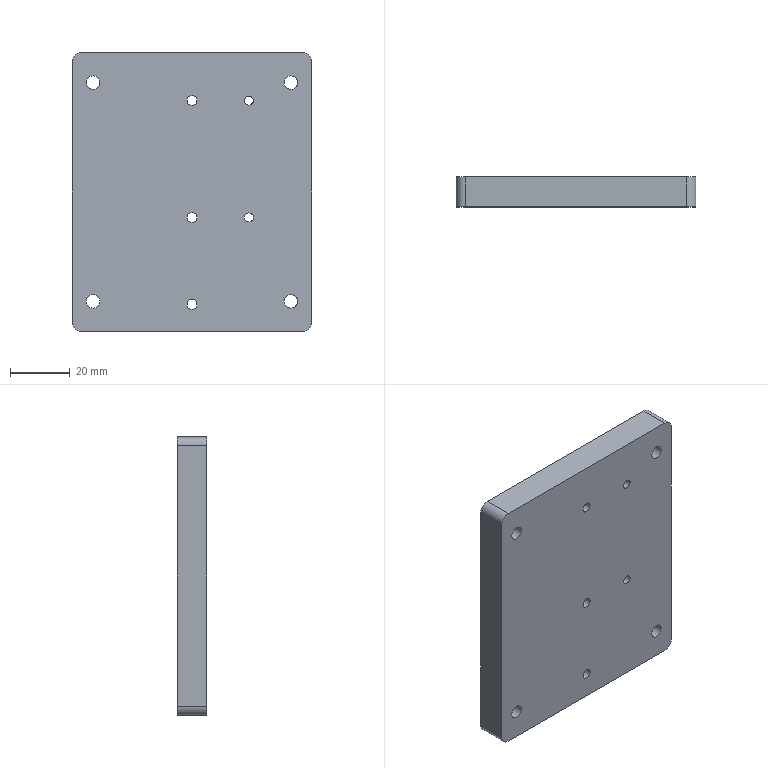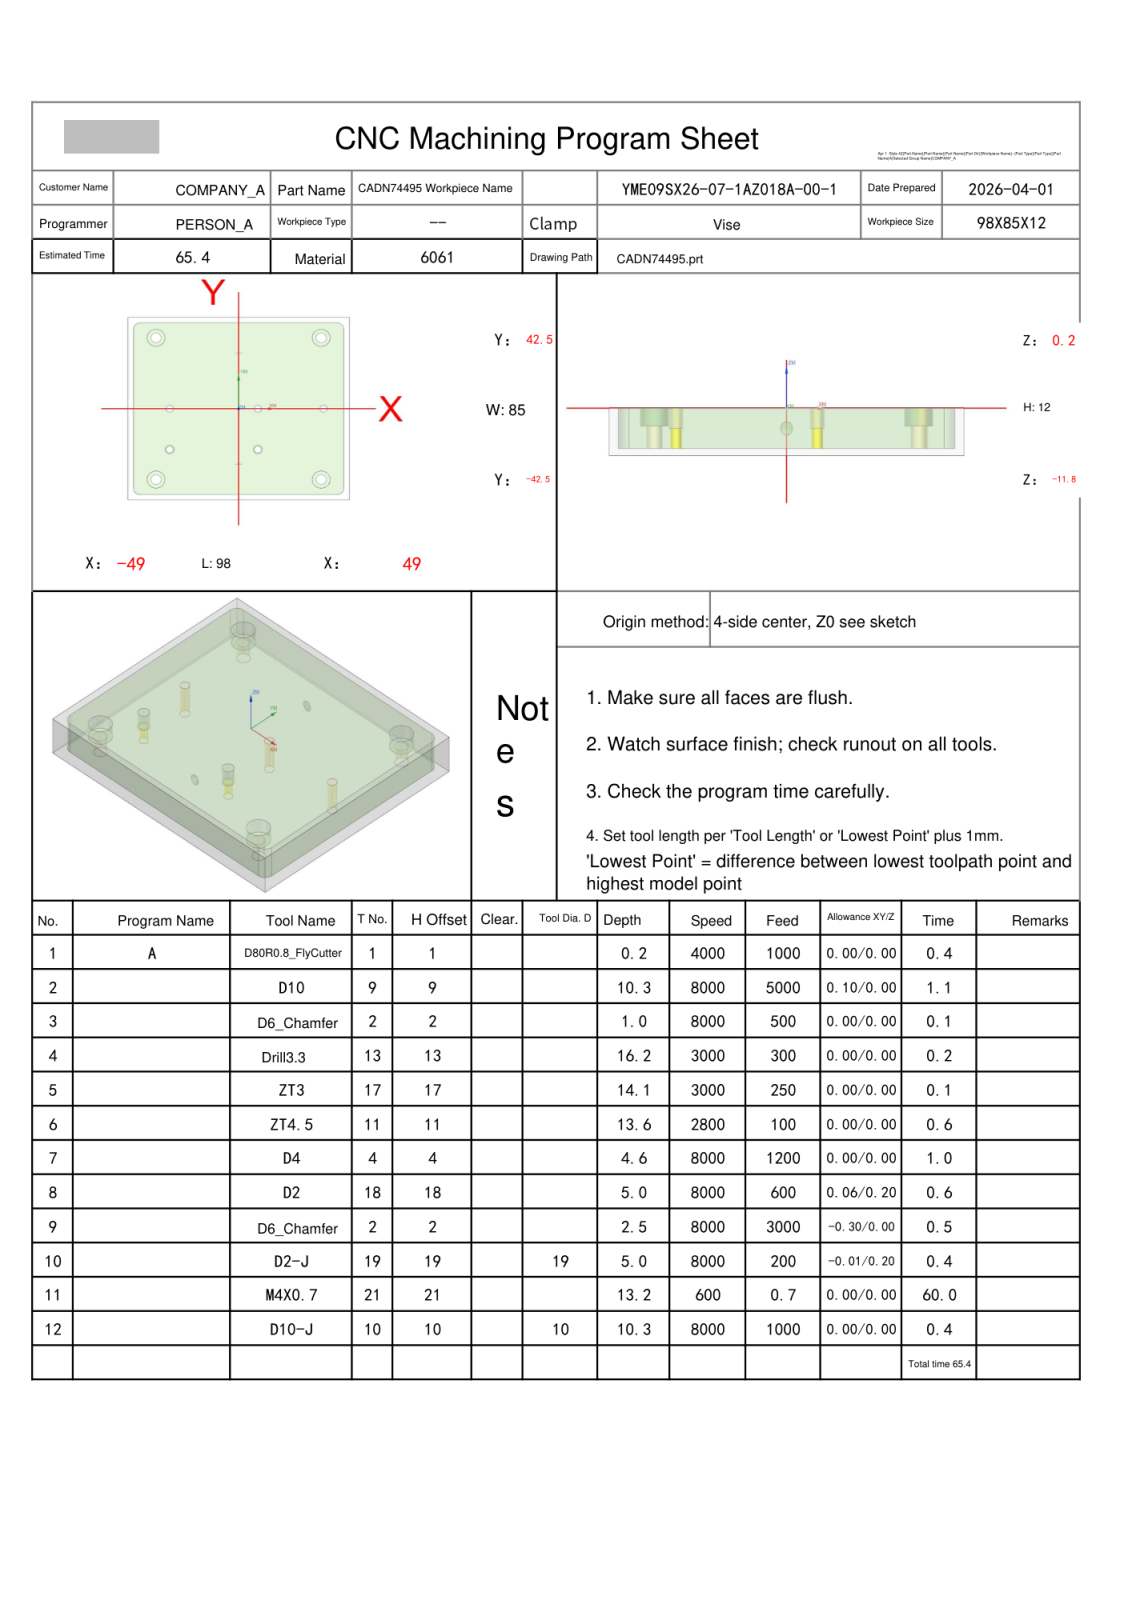NC program | NX | posted by the shop | part box 80 x 10 x 93 mm
Whole program:
%
O0001
(Machine time: 123.54 MIN)
(===Total Tool:11===)
(T1=D80R0.8 FlyCutter D=80.  R=0.8  D-  H01 Z=0.    )
(T9=D10     D=10.  R=0.   D-  H09 Z=-10.1 )
(T2=D6_Chamfer   D=6.   R=0.   D-  H02 Z=-2.3  )
(T13=Drill 3.3  D=3.3  DR_a=118 D-  H13 Z=-15.99)
(T17=ZT3    D=3.   DR_a=118 D-  H17 Z=-13.9 )
(T11=ZT4.5  D=4.5  DR_a=118 D-  H11 Z=-13.35)
(T4=D4      D=4.   R=0.   D4  H04 Z=-4.4  )
(T18=D2     D=2.   R=0.   D-  H18 Z=-4.8  )
(T19=D2-J   D=2.   R=0.   D19 H19 Z=-4.8  )
(T21=M4X0.7 D=3.3  DR_a=180 D-  H21 Z=-13.  )
(T10=D10-J  D=10.  R=0.   D10 H10 Z=-10.1 )
G80 G90 G17 G49 G40
G91 G28 Z0
M01
N1 T01 M06
(D80R0.8 FlyCutter  D=80. R=0.8 H=01 ce=0.00 di=0.00)
G00 G90 G54 X-91.5 Y26.667 M03 S4000
G43 H01 Z20.
M08
Z2.
G01 Z0.0 F1000.
X-86.5
X86.5
Y-26.667
X-86.5
X-91.5
Z2.
G00 Z20.
G91 G28 Z0.0
M05
M09
G91 G28 Z0.0
M01
N2 T09 M06
(D10  D=10. R=0. H=09 ce=0.10 di=0.00)
G00 G90 G54 X0.0 Y45.1 M03 S8000
G43 H09 Z20.
M08
Z.5
G01 X43.5 Z.412 F5000.
G02 X51.6 Y37. Z.386 I0.0 J-8.1
G01 Y-37. Z.236
G02 X43.5 Y-45.1 Z.21 I-8.1 J0.0
G01 X-43.5 Z.033
G02 X-51.6 Y-37. Z.007 I0.0 J8.1
G01 Y37. Z-.143
G02 X-43.5 Y45.1 Z-.169 I8.1 J0.0
G01 X43.5 Z-.345
G02 X51.6 Y37. Z-.371 I0.0 J-8.1
G01 Y-37. Z-.522
G02 X43.5 Y-45.1 Z-.547 I-8.1 J0.0
G01 X-43.5 Z-.724
G02 X-51.6 Y-37. Z-.75 I0.0 J8.1
G01 Y37. Z-.9
G02 X-43.5 Y45.1 Z-.926 I8.1 J0.0
G01 X43.5 Z-1.103
G02 X51.6 Y37. Z-1.128 I0.0 J-8.1
G01 Y-37. Z-1.279
G02 X43.5 Y-45.1 Z-1.305 I-8.1 J0.0
G01 X-43.5 Z-1.481
G02 X-51.6 Y-37. Z-1.507 I0.0 J8.1
G01 Y37. Z-1.657
G02 X-43.5 Y45.1 Z-1.683 I8.1 J0.0
G01 X43.5 Z-1.86
G02 X51.6 Y37. Z-1.886 I0.0 J-8.1
G01 Y-37. Z-2.036
G02 X43.5 Y-45.1 Z-2.062 I-8.1 J0.0
G01 X-43.5 Z-2.238
G02 X-51.6 Y-37. Z-2.264 I0.0 J8.1
G01 Y37. Z-2.414
G02 X-43.5 Y45.1 Z-2.44 I8.1 J0.0
G01 X43.5 Z-2.617
G02 X51.6 Y37. Z-2.643 I0.0 J-8.1
G01 Y-37. Z-2.793
G02 X43.5 Y-45.1 Z-2.819 I-8.1 J0.0
G01 X-43.5 Z-2.995
G02 X-51.6 Y-37. Z-3.021 I0.0 J8.1
G01 Y37. Z-3.172
G02 X-43.5 Y45.1 Z-3.197 I8.1 J0.0
G01 X43.5 Z-3.374
G02 X51.6 Y37. Z-3.4 I0.0 J-8.1
G01 Y-37. Z-3.55
G02 X43.5 Y-45.1 Z-3.576 I-8.1 J0.0
G01 X-43.5 Z-3.753
G02 X-51.6 Y-37. Z-3.778 I0.0 J8.1
G01 Y37. Z-3.929
G02 X-43.5 Y45.1 Z-3.955 I8.1 J0.0
G01 X43.5 Z-4.131
G02 X51.6 Y37. Z-4.157 I0.0 J-8.1
G01 Y-37. Z-4.307
G02 X43.5 Y-45.1 Z-4.333 I-8.1 J0.0
G01 X-43.5 Z-4.51
G02 X-51.6 Y-37. Z-4.536 I0.0 J8.1
G01 Y37. Z-4.686
G02 X-43.5 Y45.1 Z-4.712 I8.1 J0.0
G01 X43.5 Z-4.888
G02 X51.6 Y37. Z-4.914 I0.0 J-8.1
G01 Y-37. Z-5.064
G02 X43.5 Y-45.1 Z-5.09 I-8.1 J0.0
G01 X-43.5 Z-5.267
G02 X-51.6 Y-37. Z-5.293 I0.0 J8.1
G01 Y37. Z-5.443
G02 X-43.5 Y45.1 Z-5.469 I8.1 J0.0
G01 X43.5 Z-5.645
G02 X51.6 Y37. Z-5.671 I0.0 J-8.1
G01 Y-37. Z-5.822
G02 X43.5 Y-45.1 Z-5.847 I-8.1 J0.0
G01 X-43.5 Z-6.024
G02 X-51.6 Y-37. Z-6.05 I0.0 J8.1
G01 Y37. Z-6.2
G02 X-43.5 Y45.1 Z-6.226 I8.1 J0.0
G01 X43.5 Z-6.403
G02 X51.6 Y37. Z-6.428 I0.0 J-8.1
G01 Y-37. Z-6.579
G02 X43.5 Y-45.1 Z-6.605 I-8.1 J0.0
G01 X-43.5 Z-6.781
G02 X-51.6 Y-37. Z-6.807 I0.0 J8.1
G01 Y37. Z-6.957
G02 X-43.5 Y45.1 Z-6.983 I8.1 J0.0
G01 X43.5 Z-7.16
G02 X51.6 Y37. Z-7.186 I0.0 J-8.1
G01 Y-37. Z-7.336
G02 X43.5 Y-45.1 Z-7.362 I-8.1 J0.0
G01 X-43.5 Z-7.538
G02 X-51.6 Y-37. Z-7.564 I0.0 J8.1
G01 Y37. Z-7.714
G02 X-43.5 Y45.1 Z-7.74 I8.1 J0.0
G01 X43.5 Z-7.917
G02 X51.6 Y37. Z-7.943 I0.0 J-8.1
G01 Y-37. Z-8.093
G02 X43.5 Y-45.1 Z-8.119 I-8.1 J0.0
G01 X-43.5 Z-8.295
G02 X-51.6 Y-37. Z-8.321 I0.0 J8.1
G01 Y37. Z-8.472
G02 X-43.5 Y45.1 Z-8.497 I8.1 J0.0
G01 X43.5 Z-8.674
G02 X51.6 Y37. Z-8.7 I0.0 J-8.1
G01 Y-37. Z-8.85
G02 X43.5 Y-45.1 Z-8.876 I-8.1 J0.0
G01 X-43.5 Z-9.053
G02 X-51.6 Y-37. Z-9.078 I0.0 J8.1
G01 Y37. Z-9.229
G02 X-43.5 Y45.1 Z-9.255 I8.1 J0.0
G01 X43.5 Z-9.431
G02 X51.6 Y37. Z-9.457 I0.0 J-8.1
G01 Y-37. Z-9.607
G02 X43.5 Y-45.1 Z-9.633 I-8.1 J0.0
G01 X-43.5 Z-9.81
G02 X-51.6 Y-37. Z-9.836 I0.0 J8.1
G01 Y37. Z-9.986
G02 X-43.5 Y45.1 Z-10.012 I8.1 J0.0
G01 X0.0 Z-10.1
X43.5
G02 X51.6 Y37. I0.0 J-8.1
G01 Y-37.
G02 X43.5 Y-45.1 I-8.1 J0.0
G01 X-43.5
G02 X-51.6 Y-37. I0.0 J8.1
G01 Y37.
G02 X-43.5 Y45.1 I8.1 J0.0
G01 X0.0
X.5
Z-9.1
G00 Z20.
G91 G28 Z0.0
M05
M09
G91 G28 Z0.0
M01
N3 T02 M06
(D6_Chamfer  D=6. R=0. H=02 ce=0.00 di=0.00)
G00 G90 G54 X-36.5 Y33. M03 S8000
G43 H02 Z20.
M08
G98 G81 X-36.5 Y33. Z-.8 R1. F500.
X-30.5 Y0.0
Y-19.
X-36.5 Y-33.
X8.5 Y0.0
Y-19.
X36.5 Y-33.
X37.5 Y0.0
X36.5 Y33.
G80
G00 Z20.
G91 G28 Z0.0
M05
M09
G91 G28 Z0.0
M01
N4 T13 M06
(Drill 3.3 D=3.3 DR_a=118 H=13)
G00 G90 G54 X-30.5 Y0.0 M03 S3000
G43 H13 Z20.
M08
G98 G83 X-30.5 Y0.0 Z-15.991 R1. F300. Q2.
X8.5
X37.5
G80
G00 Z20.
G91 G28 Z0.0
M05
M09
G91 G28 Z0.0
M01
N5 T17 M06
(ZT3 D=3. DR_a=118 H=17)
G00 G90 G54 X8.5 Y-19. M03 S3000
G43 H17 Z20.
M08
G98 G83 X8.5 Y-19. Z-13.901 R1. F250. Q2.
X-30.5
G80
G00 Z20.
G91 G28 Z0.0
M05
M09
G91 G28 Z0.0
M01
N6 T11 M06
(ZT4.5 D=4.5 DR_a=118 H=11)
G00 G90 G54 X36.5 Y33. M03 S2800
G43 H11 Z20.
M08
G98 G83 X36.5 Y33. Z-13.352 R1. F100. Q2.
Y-33.
X-36.5
Y33.
G80
G00 Z20.
G91 G28 Z0.0
M05
M09
G91 G28 Z0.0
M01
N7 T04 M06
(D4  D=4. R=0. H=04 ce=0.10 di=0.00)
G00 G90 G54 X36.5 Y33. M03 S8000
G43 H04 Z20.
M08
Z.5
G03 X35.55 Y33.95 I-.95 J0.0 F1200.
X34.6 Y33. I0.0 J-.95
X34.6 Y33. Z.2 I1.9 J0.0
X34.6 Y33. Z-.1 I1.9 J0.0
X34.6 Y33. Z-.4 I1.9 J0.0
X34.6 Y33. Z-.7 I1.9 J0.0
X34.6 Y33. Z-1. I1.9 J0.0
X34.6 Y33. Z-1.3 I1.9 J0.0
X34.6 Y33. Z-1.6 I1.9 J0.0
X34.6 Y33. Z-1.9 I1.9 J0.0
X34.6 Y33. Z-2.2 I1.9 J0.0
X34.6 Y33. Z-2.5 I1.9 J0.0
X34.6 Y33. Z-2.8 I1.9 J0.0
X34.6 Y33. Z-3.1 I1.9 J0.0
X34.6 Y33. Z-3.4 I1.9 J0.0
X34.6 Y33. Z-3.7 I1.9 J0.0
X34.6 Y33. Z-4. I1.9 J0.0
X34.6 Y33. Z-4.3 I1.9 J0.0
X37.45 Y31.355 Z-4.4 I1.9 J0.0
X38.4 Y33. I-.95 J1.645
X36.5 Y34.9 I-1.9 J0.0
X34.6 Y33. I0.0 J-1.9
X36.5 Y31.1 I1.9 J0.0
X37.45 Y31.355 I0.0 J1.9
X37.925 Y32.177 I-.475 J.823
X36.975 Y33.127 I-.95 J0.0
X36.5 Y33. I0.0 J-.95
G00 Z20.
Y-33.
Z.5
G03 X35.55 Y-32.05 I-.95 J0.0
X34.6 Y-33. I0.0 J-.95
X34.6 Y-33. Z.2 I1.9 J0.0
X34.6 Y-33. Z-.1 I1.9 J0.0
X34.6 Y-33. Z-.4 I1.9 J0.0
X34.6 Y-33. Z-.7 I1.9 J0.0
X34.6 Y-33. Z-1. I1.9 J0.0
X34.6 Y-33. Z-1.3 I1.9 J0.0
X34.6 Y-33. Z-1.6 I1.9 J0.0
X34.6 Y-33. Z-1.9 I1.9 J0.0
X34.6 Y-33. Z-2.2 I1.9 J0.0
X34.6 Y-33. Z-2.5 I1.9 J0.0
X34.6 Y-33. Z-2.8 I1.9 J0.0
X34.6 Y-33. Z-3.1 I1.9 J0.0
X34.6 Y-33. Z-3.4 I1.9 J0.0
X34.6 Y-33. Z-3.7 I1.9 J0.0
X34.6 Y-33. Z-4. I1.9 J0.0
X34.6 Y-33. Z-4.3 I1.9 J0.0
X37.45 Y-34.646 Z-4.4 I1.9 J0.0
X38.4 Y-33. I-.95 J1.645
X36.5 Y-31.1 I-1.9 J0.0
X34.6 Y-33. I0.0 J-1.9
X36.5 Y-34.9 I1.9 J0.0
X37.45 Y-34.646 I0.0 J1.9
X37.925 Y-33.823 I-.475 J.823
X36.975 Y-32.873 I-.95 J0.0
X36.5 Y-33. I0.0 J-.95
G00 Z20.
X-36.5
Z.5
G03 X-37.45 Y-32.05 I-.95 J0.0
X-38.4 Y-33. I0.0 J-.95
X-38.4 Y-33. Z.2 I1.9 J0.0
X-38.4 Y-33. Z-.1 I1.9 J0.0
X-38.4 Y-33. Z-.4 I1.9 J0.0
X-38.4 Y-33. Z-.7 I1.9 J0.0
X-38.4 Y-33. Z-1. I1.9 J0.0
X-38.4 Y-33. Z-1.3 I1.9 J0.0
X-38.4 Y-33. Z-1.6 I1.9 J0.0
X-38.4 Y-33. Z-1.9 I1.9 J0.0
X-38.4 Y-33. Z-2.2 I1.9 J0.0
X-38.4 Y-33. Z-2.5 I1.9 J0.0
X-38.4 Y-33. Z-2.8 I1.9 J0.0
X-38.4 Y-33. Z-3.1 I1.9 J0.0
X-38.4 Y-33. Z-3.4 I1.9 J0.0
X-38.4 Y-33. Z-3.7 I1.9 J0.0
X-38.4 Y-33. Z-4. I1.9 J0.0
X-38.4 Y-33. Z-4.3 I1.9 J0.0
X-35.55 Y-34.646 Z-4.4 I1.9 J0.0
X-34.6 Y-33. I-.95 J1.645
X-36.5 Y-31.1 I-1.9 J0.0
X-38.4 Y-33. I0.0 J-1.9
X-36.5 Y-34.9 I1.9 J0.0
X-35.55 Y-34.646 I0.0 J1.9
X-35.075 Y-33.823 I-.475 J.823
X-36.025 Y-32.873 I-.95 J0.0
X-36.5 Y-33. I0.0 J-.95
G00 Z20.
Y33.
Z.5
G03 X-37.45 Y33.95 I-.95 J0.0
X-38.4 Y33. I0.0 J-.95
X-38.4 Y33. Z.2 I1.9 J0.0
X-38.4 Y33. Z-.1 I1.9 J0.0
X-38.4 Y33. Z-.4 I1.9 J0.0
X-38.4 Y33. Z-.7 I1.9 J0.0
X-38.4 Y33. Z-1. I1.9 J0.0
X-38.4 Y33. Z-1.3 I1.9 J0.0
X-38.4 Y33. Z-1.6 I1.9 J0.0
X-38.4 Y33. Z-1.9 I1.9 J0.0
X-38.4 Y33. Z-2.2 I1.9 J0.0
X-38.4 Y33. Z-2.5 I1.9 J0.0
X-38.4 Y33. Z-2.8 I1.9 J0.0
X-38.4 Y33. Z-3.1 I1.9 J0.0
X-38.4 Y33. Z-3.4 I1.9 J0.0
X-38.4 Y33. Z-3.7 I1.9 J0.0
X-38.4 Y33. Z-4. I1.9 J0.0
X-38.4 Y33. Z-4.3 I1.9 J0.0
X-35.55 Y31.355 Z-4.4 I1.9 J0.0
X-34.6 Y33. I-.95 J1.645
X-36.5 Y34.9 I-1.9 J0.0
X-38.4 Y33. I0.0 J-1.9
X-36.5 Y31.1 I1.9 J0.0
X-35.55 Y31.355 I0.0 J1.9
X-35.075 Y32.177 I-.475 J.823
X-36.025 Y33.127 I-.95 J0.0
X-36.5 Y33. I0.0 J-.95
G00 Z20.
G00 G90 X36.5 Y33. M03 S8000
Z20.
Z.5
G41 D04
G01 X36.46 Y33.196 F500.
G03 X35.49 Y33.99 I-.97 J-.196
X34.5 Y33. I0.0 J-.99
X34.516 Y33.251 Z-4.4 I2. J0.0
X34.5 Y33. I1.984 J-.251
X36.5 Y31. I2. J0.0
X38.5 Y33. I0.0 J2.
X36.5 Y35. I-2. J0.0
X34.516 Y33.251 I0.0 J-2.
G01 X34.508 Y33.127
G03 X35.498 Y32.137 I.99 J0.0
X36.436 Y32.81 I0.0 J.99
G01 G40 X36.5 Y33.
G00 Z20.
Y-33.
Z.5
G41 D04
G01 X36.46 Y-32.804
G03 X35.49 Y-32.01 I-.97 J-.196
X34.5 Y-33. I0.0 J-.99
X34.516 Y-32.749 Z-4.4 I2. J0.0
X34.5 Y-33. I1.984 J-.251
X36.5 Y-35. I2. J0.0
X38.5 Y-33. I0.0 J2.
X36.5 Y-31. I-2. J0.0
X34.516 Y-32.749 I0.0 J-2.
G01 X34.508 Y-32.873
G03 X35.498 Y-33.863 I.99 J0.0
X36.436 Y-33.19 I0.0 J.99
G01 G40 X36.5 Y-33.
G00 Z20.
X-36.5
Z.5
G41 D04
G01 X-36.54 Y-32.804
G03 X-37.51 Y-32.01 I-.97 J-.196
X-38.5 Y-33. I0.0 J-.99
X-38.484 Y-32.749 Z-4.4 I2. J0.0
X-38.5 Y-33. I1.984 J-.251
X-36.5 Y-35. I2. J0.0
X-34.5 Y-33. I0.0 J2.
X-36.5 Y-31. I-2. J0.0
X-38.484 Y-32.749 I0.0 J-2.
G01 X-38.492 Y-32.873
G03 X-37.502 Y-33.863 I.99 J0.0
X-36.564 Y-33.19 I0.0 J.99
G01 G40 X-36.5 Y-33.
G00 Z20.
Y33.
Z.5
G41 D04
G01 X-36.54 Y33.196
G03 X-37.51 Y33.99 I-.97 J-.196
X-38.5 Y33. I0.0 J-.99
X-38.484 Y33.251 Z-4.4 I2. J0.0
X-38.5 Y33. I1.984 J-.251
X-36.5 Y31. I2. J0.0
X-34.5 Y33. I0.0 J2.
X-36.5 Y35. I-2. J0.0
X-38.484 Y33.251 I0.0 J-2.
G01 X-38.492 Y33.127
G03 X-37.502 Y32.137 I.99 J0.0
X-36.564 Y32.81 I0.0 J.99
G01 G40 X-36.5 Y33.
G00 Z20.
G91 G28 Z0.0
M05
M09
G91 G28 Z0.0
M01
N8 T18 M06
(D2  D=2. R=0. H=18 ce=0.06 di=0.20)
G00 G90 G54 X8.5 Y-19. M03 S8000
G43 H18 Z20.
M08
Z.5
G03 X8.03 Y-18.53 I-.47 J0.0 F600.
X7.56 Y-19. I0.0 J-.47
X7.56 Y-19. Z.3 I.94 J0.0
X7.56 Y-19. Z.1 I.94 J0.0
X7.56 Y-19. Z-.1 I.94 J0.0
X7.56 Y-19. Z-.3 I.94 J0.0
X7.56 Y-19. Z-.5 I.94 J0.0
X7.56 Y-19. Z-.7 I.94 J0.0
X7.56 Y-19. Z-.9 I.94 J0.0
X7.56 Y-19. Z-1.1 I.94 J0.0
X7.56 Y-19. Z-1.3 I.94 J0.0
X7.56 Y-19. Z-1.5 I.94 J0.0
X7.56 Y-19. Z-1.7 I.94 J0.0
X7.56 Y-19. Z-1.9 I.94 J0.0
X7.56 Y-19. Z-2.1 I.94 J0.0
X7.56 Y-19. Z-2.3 I.94 J0.0
X7.56 Y-19. Z-2.5 I.94 J0.0
X7.56 Y-19. Z-2.7 I.94 J0.0
X7.56 Y-19. Z-2.9 I.94 J0.0
X7.56 Y-19. Z-3.1 I.94 J0.0
X7.56 Y-19. Z-3.3 I.94 J0.0
X7.56 Y-19. Z-3.5 I.94 J0.0
X7.56 Y-19. Z-3.7 I.94 J0.0
X7.56 Y-19. Z-3.9 I.94 J0.0
X7.56 Y-19. Z-4.1 I.94 J0.0
X7.56 Y-19. Z-4.3 I.94 J0.0
X7.56 Y-19. Z-4.5 I.94 J0.0
X7.56 Y-19. Z-4.7 I.94 J0.0
X9.44 Y-19. Z-4.8 I.94 J0.0
X8.5 Y-18.06 I-.94 J0.0
X7.56 Y-19. I0.0 J-.94
X8.5 Y-19.94 I.94 J0.0
X9.44 Y-19. I0.0 J.94
X8.97 Y-18.53 I-.47 J0.0
X8.5 Y-19. I0.0 J-.47
G00 Z20.
X-30.5
Z.5
G03 X-30.97 Y-18.53 I-.47 J0.0
X-31.44 Y-19. I0.0 J-.47
X-31.44 Y-19. Z.3 I.94 J0.0
X-31.44 Y-19. Z.1 I.94 J0.0
X-31.44 Y-19. Z-.1 I.94 J0.0
X-31.44 Y-19. Z-.3 I.94 J0.0
X-31.44 Y-19. Z-.5 I.94 J0.0
X-31.44 Y-19. Z-.7 I.94 J0.0
X-31.44 Y-19. Z-.9 I.94 J0.0
X-31.44 Y-19. Z-1.1 I.94 J0.0
X-31.44 Y-19. Z-1.3 I.94 J0.0
X-31.44 Y-19. Z-1.5 I.94 J0.0
X-31.44 Y-19. Z-1.7 I.94 J0.0
X-31.44 Y-19. Z-1.9 I.94 J0.0
X-31.44 Y-19. Z-2.1 I.94 J0.0
X-31.44 Y-19. Z-2.3 I.94 J0.0
X-31.44 Y-19. Z-2.5 I.94 J0.0
X-31.44 Y-19. Z-2.7 I.94 J0.0
X-31.44 Y-19. Z-2.9 I.94 J0.0
X-31.44 Y-19. Z-3.1 I.94 J0.0
X-31.44 Y-19. Z-3.3 I.94 J0.0
X-31.44 Y-19. Z-3.5 I.94 J0.0
X-31.44 Y-19. Z-3.7 I.94 J0.0
X-31.44 Y-19. Z-3.9 I.94 J0.0
X-31.44 Y-19. Z-4.1 I.94 J0.0
X-31.44 Y-19. Z-4.3 I.94 J0.0
X-31.44 Y-19. Z-4.5 I.94 J0.0
X-31.44 Y-19. Z-4.7 I.94 J0.0
X-29.56 Y-19. Z-4.8 I.94 J0.0
X-30.5 Y-18.06 I-.94 J0.0
X-31.44 Y-19. I0.0 J-.94
X-30.5 Y-19.94 I.94 J0.0
X-29.56 Y-19. I0.0 J.94
X-30.03 Y-18.53 I-.47 J0.0
X-30.5 Y-19. I0.0 J-.47
G00 Z20.
G91 G28 Z0.0
M05
M09
G91 G28 Z0.0
M01
N9 T02 M06
(D6_Chamfer  D=6. R=0. H=02 ce=0.00 di=0.00)
G00 G90 G54 X-.249 Y42.128 M03 S8000
G43 H02 Z20.
M08
Z2.099
G01 Z-1.499 F3000.
G03 X-.33 Y41.828 I.52 J-.3
X-.03 Y41.308 I.6 J0.0
G01 X0.0 Y41.3
X43.5
G02 X47.8 Y37. I0.0 J-4.3
G01 Y-37.
G02 X43.5 Y-41.3 I-4.3 J0.0
G01 X-43.5
G02 X-47.8 Y-37. I0.0 J4.3
G01 Y37.
G02 X-43.5 Y41.3 I4.3 J0.0
G01 X0.0
X.03 Y41.308
G03 X.33 Y41.828 I-.3 J.52
X.25 Y42.128 I-.6 J0.0
G01 Z2.099
G00 Z20.
G00 G90 X-30.5 Y0.0 M03 S8000
Z20.
G98 G81 X-30.5 Y0.0 Z-2.2 R3. F500.
X8.5
X37.5
G80
G00 Z20.
G00 G90 X8.5 Y-19. M03 S8000
Z20.
G98 G81 X8.5 Y-19. Z-2.3 R3. F500.
X-30.5
G80
G00 Z20.
G00 G90 X-39.712 Y32.253 M03 S8000
Z20.
Z2.5
G01 X-39.66 Y32.038 Z2.42 F500.
X-39.524 Y31.672 Z2.278
X-39.347 Y31.325 Z2.136
X-39.129 Y31.001 Z1.994
X-38.875 Y30.705 Z1.852
X-38.588 Y30.441 Z1.71
X-38.272 Y30.212 Z1.568
X-38.028 Y30.072 Z1.465
X-37.672 Y29.912 Z1.323
X-37.3 Y29.795 Z1.181
X-36.916 Y29.723 Z1.039
X-36.527 Y29.697 Z.897
X-36.138 Y29.717 Z.755
X-35.753 Y29.783 Z.613
X-35.379 Y29.893 Z.471
X-35.02 Y30.047 Z.329
X-34.682 Y30.242 Z.187
X-34.37 Y30.476 Z.045
X-34.087 Y30.744 Z-.097
X-33.838 Y31.045 Z-.239
X-33.626 Y31.372 Z-.381
X-33.454 Y31.722 Z-.523
X-33.325 Y32.09 Z-.665
X-33.24 Y32.471 Z-.807
X-33.2 Y32.859 Z-.949
Y33. Z-1.
G03 X-36.5 Y36.3 I-3.3 J0.0
X-39.8 Y33. I0.0 J-3.3
X-36.5 Y29.7 I3.3 J0.0
X-33.2 Y33. I0.0 J3.3
X-33.238 Y33.498 I-3.3 J0.0
G01 Z1.5
G00 Z20.
X-39.712 Y-33.747
Z2.5
G01 X-39.66 Y-33.962 Z2.42
X-39.524 Y-34.328 Z2.278
X-39.347 Y-34.675 Z2.136
X-39.129 Y-34.999 Z1.994
X-38.875 Y-35.295 Z1.852
X-38.588 Y-35.559 Z1.71
X-38.272 Y-35.788 Z1.568
X-38.028 Y-35.928 Z1.465
X-37.672 Y-36.088 Z1.323
X-37.3 Y-36.205 Z1.181
X-36.916 Y-36.277 Z1.039
X-36.527 Y-36.303 Z.897
X-36.138 Y-36.283 Z.755
X-35.753 Y-36.217 Z.613
X-35.379 Y-36.107 Z.471
X-35.02 Y-35.953 Z.329
X-34.682 Y-35.758 Z.187
X-34.37 Y-35.524 Z.045
X-34.087 Y-35.256 Z-.097
X-33.838 Y-34.955 Z-.239
X-33.626 Y-34.628 Z-.381
X-33.454 Y-34.278 Z-.523
X-33.325 Y-33.91 Z-.665
X-33.24 Y-33.529 Z-.807
X-33.2 Y-33.141 Z-.949
Y-33. Z-1.
G03 X-36.5 Y-29.7 I-3.3 J0.0
X-39.8 Y-33. I0.0 J-3.3
X-36.5 Y-36.3 I3.3 J0.0
X-33.2 Y-33. I0.0 J3.3
X-33.238 Y-32.502 I-3.3 J0.0
G01 Z1.5
G00 Z20.
X33.288 Y-33.747
Z2.5
G01 X33.34 Y-33.962 Z2.42
X33.476 Y-34.328 Z2.278
X33.653 Y-34.675 Z2.136
X33.871 Y-34.999 Z1.994
X34.125 Y-35.295 Z1.852
X34.412 Y-35.559 Z1.71
X34.728 Y-35.788 Z1.568
X34.972 Y-35.928 Z1.465
X35.328 Y-36.088 Z1.323
X35.7 Y-36.205 Z1.181
X36.084 Y-36.277 Z1.039
X36.473 Y-36.303 Z.897
X36.862 Y-36.283 Z.755
X37.247 Y-36.217 Z.613
X37.621 Y-36.107 Z.471
X37.98 Y-35.953 Z.329
X38.318 Y-35.758 Z.187
X38.63 Y-35.524 Z.045
X38.913 Y-35.256 Z-.097
X39.162 Y-34.955 Z-.239
X39.374 Y-34.628 Z-.381
X39.546 Y-34.278 Z-.523
X39.675 Y-33.91 Z-.665
X39.76 Y-33.529 Z-.807
X39.8 Y-33.141 Z-.949
Y-33. Z-1.
G03 X36.5 Y-29.7 I-3.3 J0.0
X33.2 Y-33. I0.0 J-3.3
X36.5 Y-36.3 I3.3 J0.0
X39.8 Y-33. I0.0 J3.3
X39.762 Y-32.502 I-3.3 J0.0
G01 Z1.5
G00 Z20.
X33.288 Y32.253
Z2.5
G01 X33.34 Y32.038 Z2.42
X33.476 Y31.672 Z2.278
X33.653 Y31.325 Z2.136
X33.871 Y31.001 Z1.994
X34.125 Y30.705 Z1.852
X34.412 Y30.441 Z1.71
X34.728 Y30.212 Z1.568
X34.972 Y30.072 Z1.465
X35.328 Y29.912 Z1.323
X35.7 Y29.795 Z1.181
X36.084 Y29.723 Z1.039
X36.473 Y29.697 Z.897
X36.862 Y29.717 Z.755
X37.247 Y29.783 Z.613
X37.621 Y29.893 Z.471
X37.98 Y30.047 Z.329
X38.318 Y30.242 Z.187
X38.63 Y30.476 Z.045
X38.913 Y30.744 Z-.097
X39.162 Y31.045 Z-.239
X39.374 Y31.372 Z-.381
X39.546 Y31.722 Z-.523
X39.675 Y32.09 Z-.665
X39.76 Y32.471 Z-.807
X39.8 Y32.859 Z-.949
Y33. Z-1.
G03 X36.5 Y36.3 I-3.3 J0.0
X33.2 Y33. I0.0 J-3.3
X36.5 Y29.7 I3.3 J0.0
X39.8 Y33. I0.0 J3.3
X39.762 Y33.498 I-3.3 J0.0
G01 Z1.5
G00 Z20.
G91 G28 Z0.0
M05
M09
G91 G28 Z0.0
M01
N10 T19 M06
(D2-J  D=2. R=0. H=19 ce=-0.01 di=0.20)
G00 G90 G54 X8.5 Y-19. M03 S8000
G43 H19 Z20.
M08
Z.5
G41 D19
G01 X8.424 Y-18.815 F200.
G03 X7.975 Y-18.515 I-.449 J-.185
X7.49 Y-19. I0.0 J-.485
X7.49 Y-19. Z-.5 I1.01 J0.0
X7.49 Y-19. Z-1.5 I1.01 J0.0
X7.49 Y-19. Z-2.5 I1.01 J0.0
X7.49 Y-19. Z-3.5 I1.01 J0.0
X7.49 Y-19. Z-4.5 I1.01 J0.0
X8.812 Y-19.961 Z-4.8 I1.01 J0.0
X9.51 Y-19. I-.312 J.961
X8.5 Y-17.99 I-1.01 J0.0
X7.49 Y-19. I0.0 J-1.01
X8.5 Y-20.01 I1.01 J0.0
X8.812 Y-19.961 I0.0 J1.01
X9.147 Y-19.499 I-.15 J.461
X8.699 Y-19.015 I-.485 J0.0
G01 G40 X8.5 Y-19.
G00 Z20.
X-30.5
Z.5
G41 D19
G01 X-30.576 Y-18.815
G03 X-31.025 Y-18.515 I-.449 J-.185
X-31.51 Y-19. I0.0 J-.485
X-31.51 Y-19. Z-.5 I1.01 J0.0
X-31.51 Y-19. Z-1.5 I1.01 J0.0
X-31.51 Y-19. Z-2.5 I1.01 J0.0
X-31.51 Y-19. Z-3.5 I1.01 J0.0
X-31.51 Y-19. Z-4.5 I1.01 J0.0
X-30.188 Y-19.961 Z-4.8 I1.01 J0.0
X-29.49 Y-19. I-.312 J.961
X-30.5 Y-17.99 I-1.01 J0.0
X-31.51 Y-19. I0.0 J-1.01
X-30.5 Y-20.01 I1.01 J0.0
X-30.188 Y-19.961 I0.0 J1.01
X-29.853 Y-19.499 I-.15 J.461
X-30.301 Y-19.015 I-.485 J0.0
G01 G40 X-30.5 Y-19.
G00 Z20.
G91 G28 Z0.0
M05
M09
G91 G28 Z0.0
M01
N11 T21 M06
(M4X0.7 D=3.3 DR_a=180 H=21)
G00 G90 G54 X-30.5 Y0.0 M03 S600
G43 H21 Z20.
M08
G95
G98 G84 X-30.5 Y0.0 Z-13. R1. F.7 Q4.
X8.5
X37.5
G80
G94
G00 Z20.
G91 G28 Z0.0
M05
M09
G91 G28 Z0.0
M01
N12 T10 M06
(D10-J  D=10. R=0. H=10 ce=0.00 di=0.00)
G00 G90 G54 X44.51 Y-46.144 M03 S8000
G43 H10 Z20.
M08
Z-9.6
G01 Z-10.1 F1000.
G41 D10
X44.498 Y-45.944
G03 X43.5 Y-45. I-.998 J-.056
G01 X-43.5
G02 X-51.5 Y-37. I0.0 J8.
G01 Y37.
G02 X-43.5 Y45. I8. J0.0
G01 X43.5
G02 X51.5 Y37. I0.0 J-8.
G01 Y-37.
G02 X43.5 Y-45. I-8. J0.0
G01 X43.
G03 X42. Y-46. I0.0 J-1.
G01 G40 Y-46.2
Z-9.6
G00 Z20.
M05
M09
G91 G28 Z0.0
G91 G28 Y0.0
M30
%